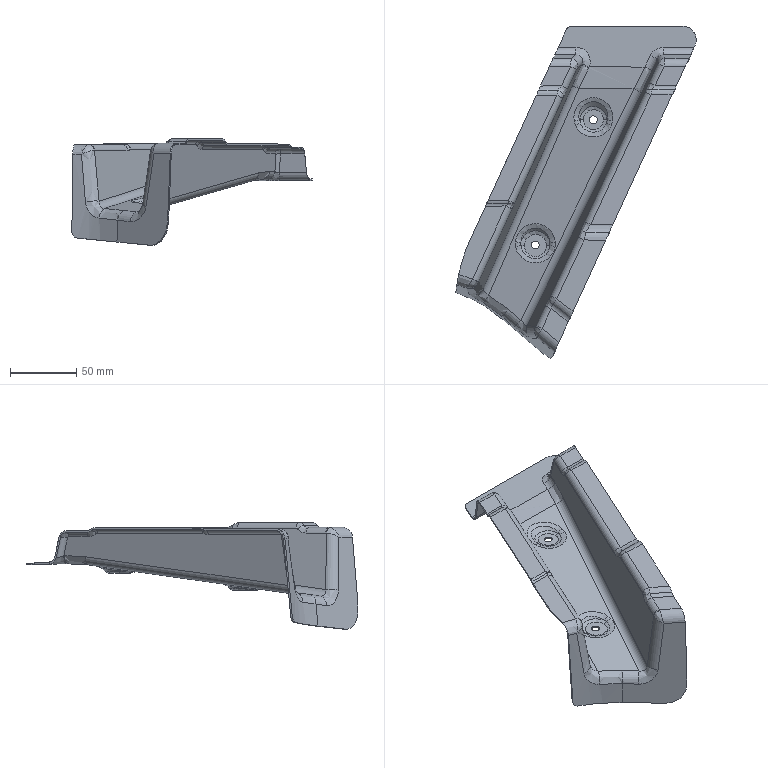Part | 1 solid | 221 faces | box 181.011 x 250 x 80.326 mm | volume 46704 mm3 | spline 123 | cylinder 63 | plane 31 | other 2 | sphere 2 | commonest cylinder face diameters 10 x13 7.6 x9 12 x7 14.4 x5 6 x4 12.4 x4